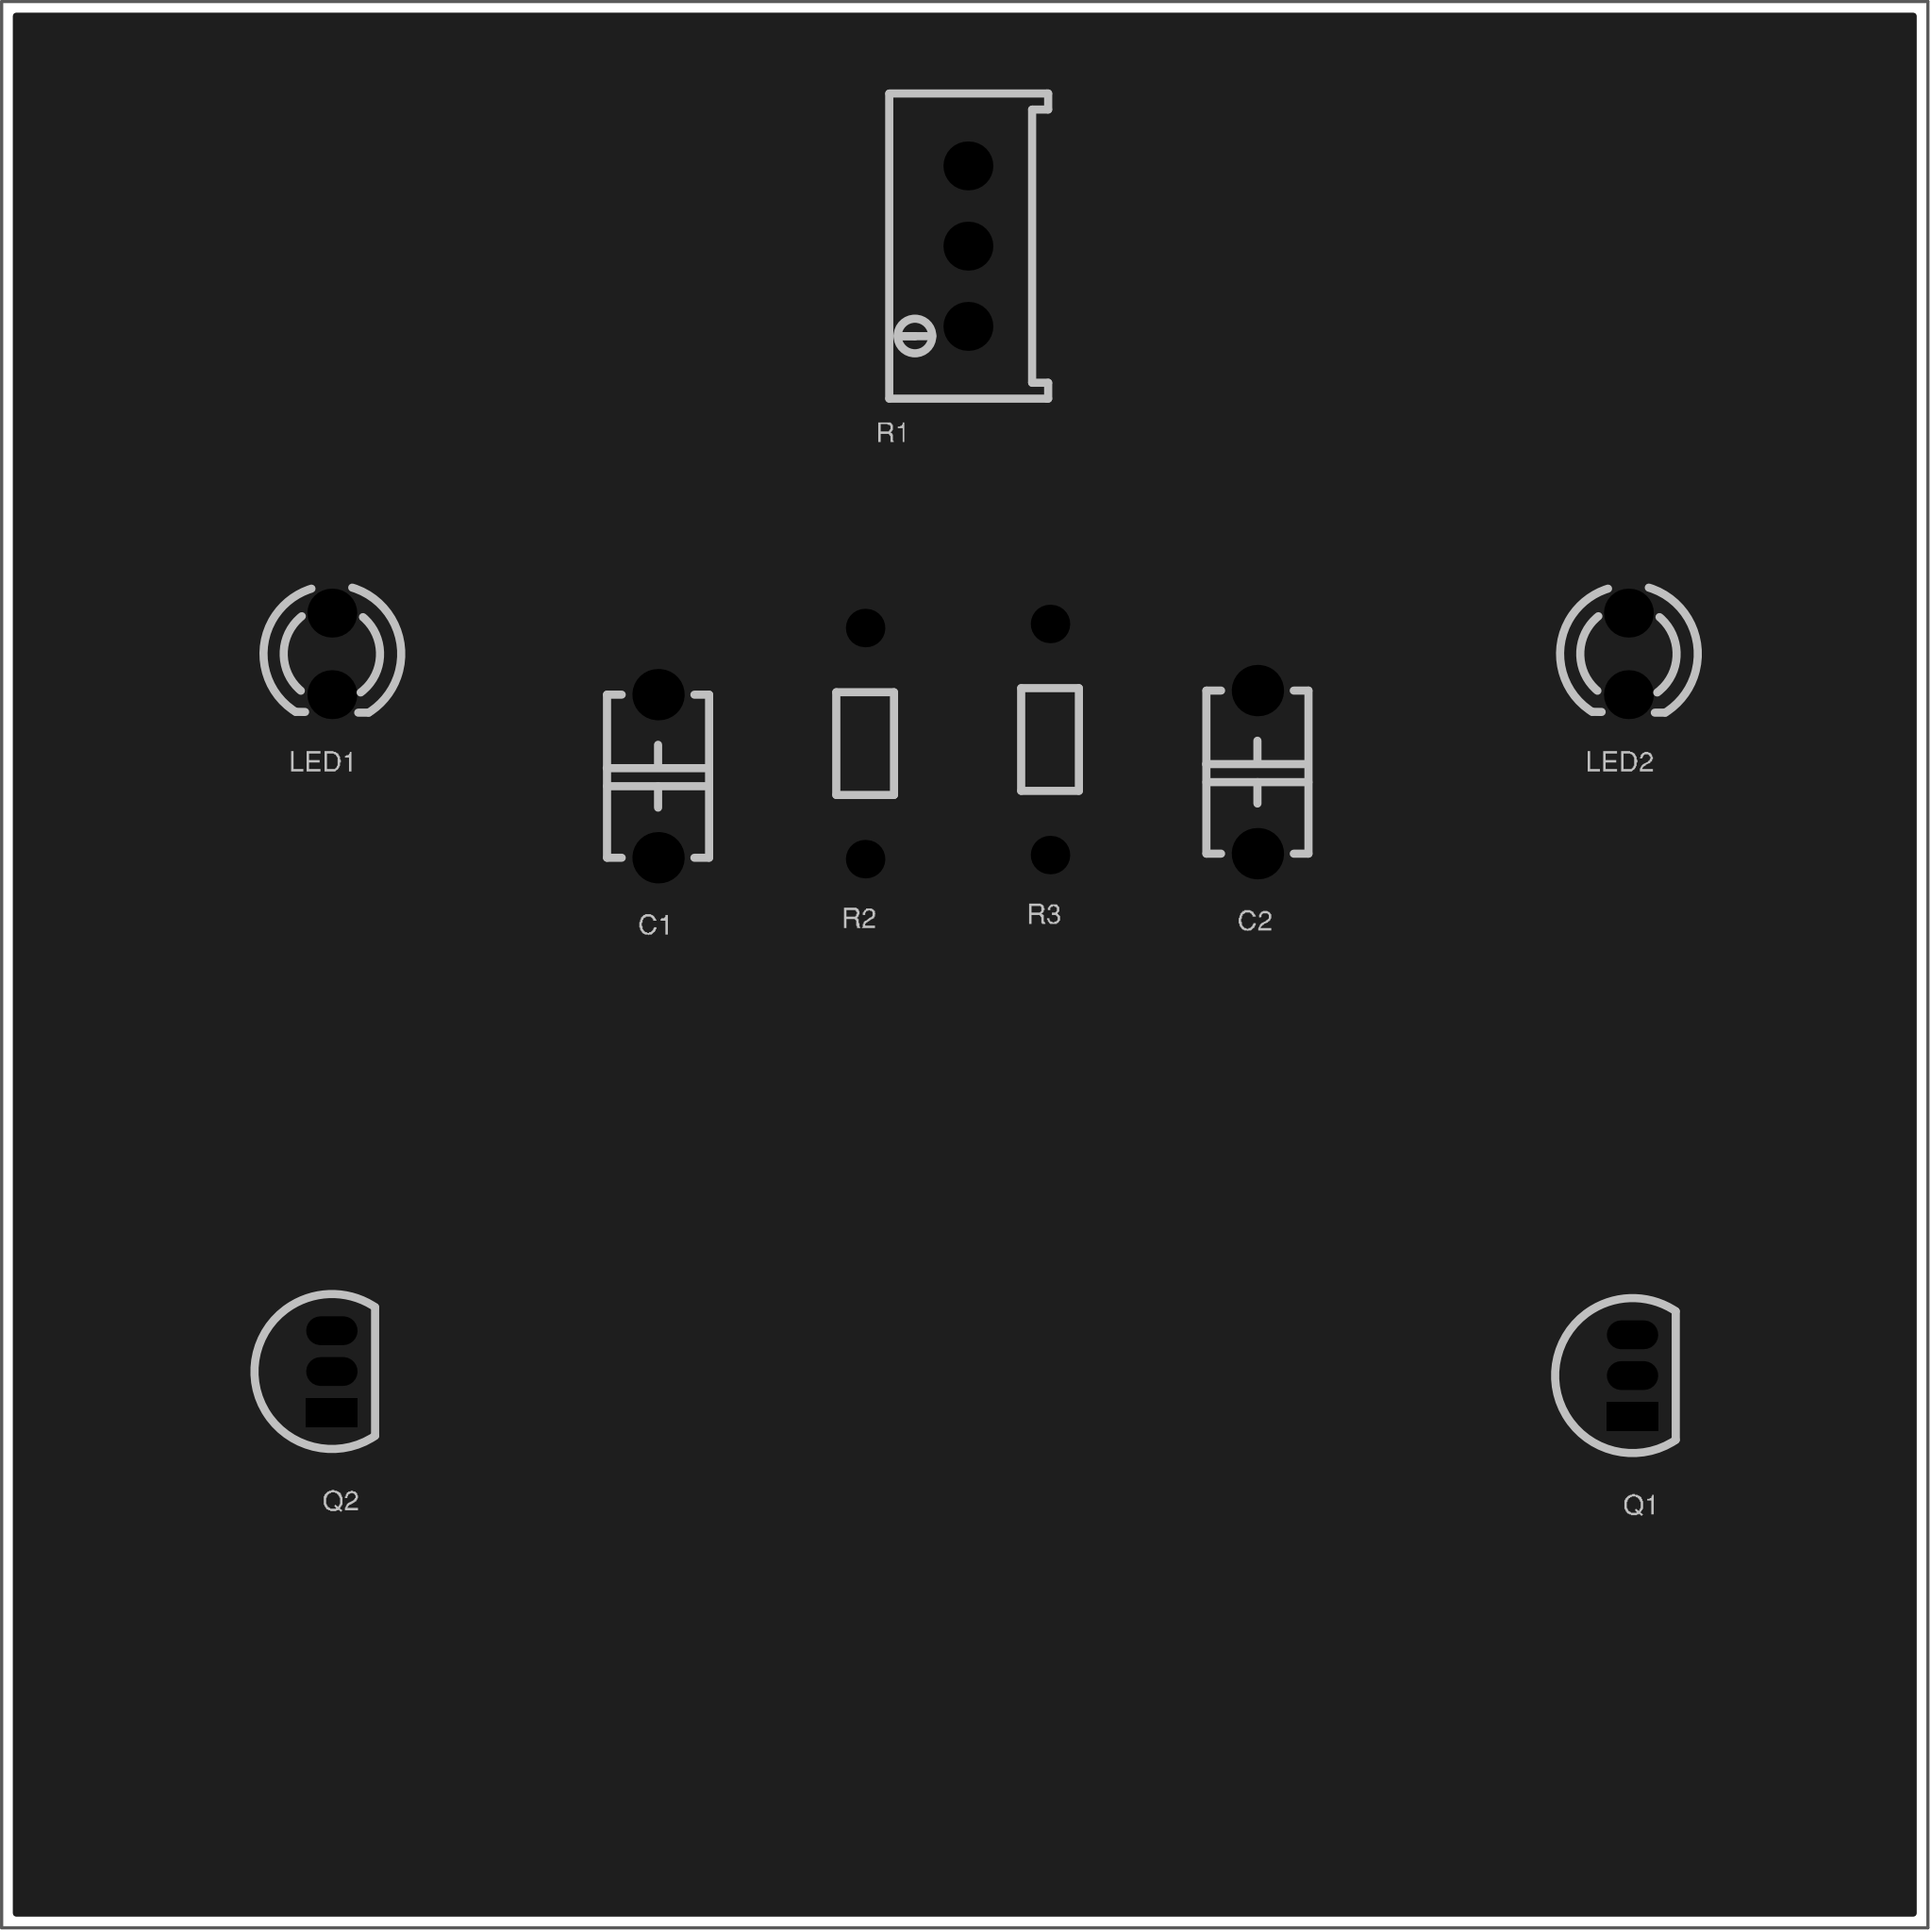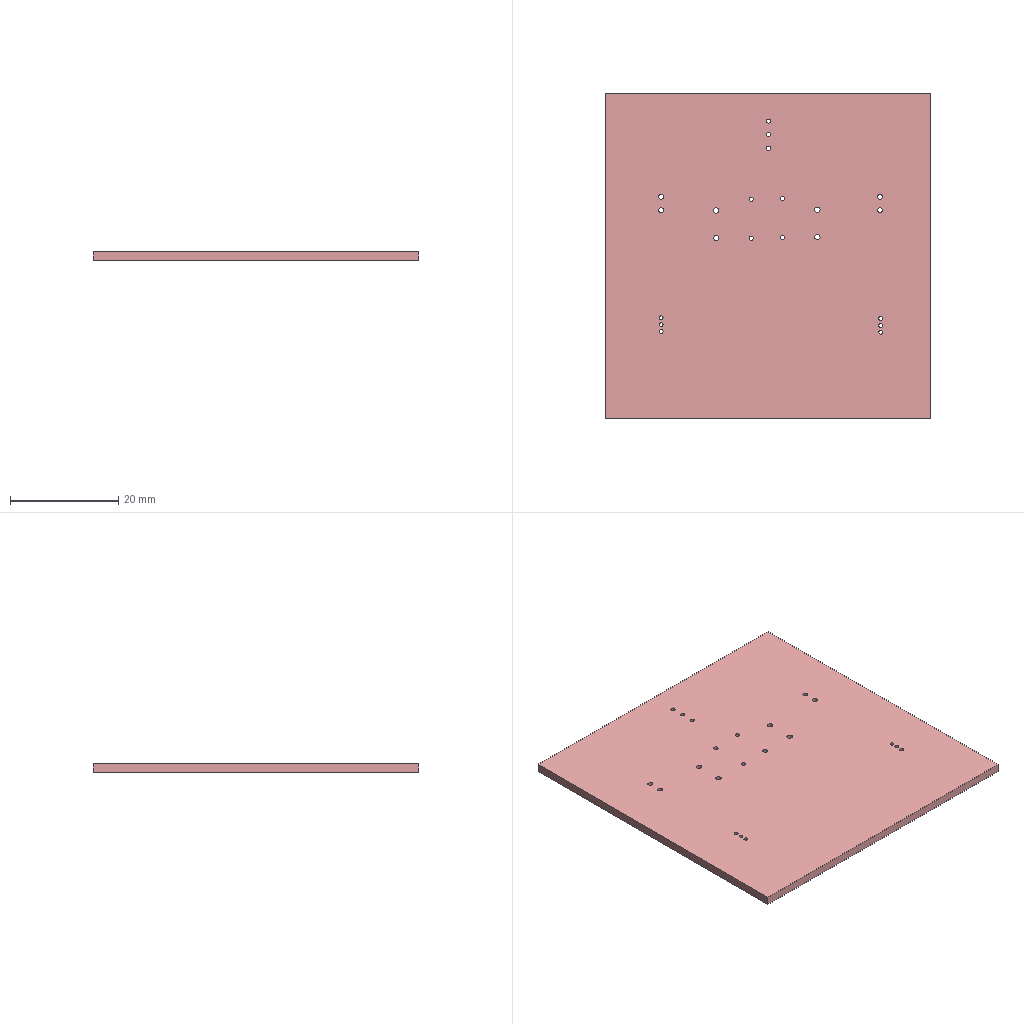Circuit board layout | Altium Designer | box 60 x 60 x 1.6 mm
Layer stack:
# Altium Designer layer stack of  (unit mm; dielectric type: 0 none, 1 core, 2 prepreg, 3 surface material)
index,name,kind,layer,copper_thickness_mm,dielectric_type,dielectric_thickness_mm,dielectric_material,dielectric_constant
0,Top Paste Mask Layer,other,,,,,,
1,Top Silkscreen Layer,other,,,,,,
2,Top Solder Mask Layer,dielectric,,,3,0.01,,3.3
3,Top Layer,copper,Top Layer,0.035,,,,
4,Dielectric1,dielectric,,,3,1.51,FR4,4.5
5,Bottom Layer,copper,Bottom Layer,0.035,,,,
6,Bottom Solder Mask Layer,dielectric,,,3,0.01,,3.3
7,Bottom Silkscreen Layer,other,,,,,,
8,Bottom Paste Mask Layer,other,,,,,,
# drill layer pairs: low layer,high layer
drill_pair,Top Layer,Bottom Layer
Part placement:
Designator,Comment,Layer,Footprint,Center-X(mm),Center-Y(mm),Rotation
C1,100uF,TopLayer,CAP-TH_L5.1-W3.2-P5.08-D0.50,96.647,112.07,270
C2,100uF,TopLayer,CAP-TH_L5.1-W3.2-P5.08-D0.50,115.316,112.197,270
LED1,,TopLayer,LED_TH-3mm,86.487,115.88,270
LED2,,TopLayer,LED_TH-3mm,126.873,115.88,270
Q1,,TopLayer,S8050_TO_92,127,93.401,90
Q2,,TopLayer,S8050_TO_92,86.487,93.528,90
R1,10k,TopLayer,R_3296,106.299,128.58,90
R2,10k,TopLayer,Res_1/8W,103.097,113.086,90
R3,10k,TopLayer,Res_1/8W,108.856,113.213,90
Pad and via stacks:
# Altium Designer via and pad stacks of  (unit mm). Each distinct definition once, with the count of objects using it.
# via: kind,start_layer,end_layer,hole_mm,diameter_mm,mode(0 simple;1 top-mid-bottom;2 full stack),diameter_per_layer,count,example_net
# pad: kind,layer,hole_mm,hole_type(0 round;1 square;2 slot),plating,top_size,top_shape(1 round;2 rect;3 octagon;9 rounded rect),mid_size,bottom_size,mode,footprint,size_per_layer,count,example
pad,Multi-Layer,1,0,plated,1.6x1.6,1,1.6x1.6,1.6x1.6,0,CAP-TH_L5.1-W3.2-P5.08-D0.50,,4,C1.2
pad,Multi-Layer,0.9144,0,plated,1.524x1.524,1,1.524x1.524,1.524x1.524,0,LED_TH-3mm,,4,LED1.1
pad,Multi-Layer,0.701,0,plated,0.8992x1.6,2,0.8992x1.6,0.8992x1.6,0,S8050_TO_92,,2,Q1.1
pad,Multi-Layer,0.701,0,plated,0.8992x1.6,1,0.8992x1.6,0.8992x1.6,0,S8050_TO_92,,4,Q1.2
pad,Multi-Layer,0.762,0,plated,1.524x1.524,1,1.524x1.524,1.524x1.524,0,R_3296,,3,R1.2
pad,Multi-Layer,0.8001,0,plated,1.199x1.199,1,1.199x1.199,1.199x1.199,0,Res_1/8W,,4,R2.1
Copper pours:
name,layer,net,type(0 solid;1 hatched;2 none)
Top Layer-GND,Top Layer,GND,0
Bottom Layer-GND,Bottom Layer,GND,0
Design rules, without the lines most boards share:
# Altium Designer design rules of  (exported by Altium Designer, unit mm)
# columns: name | kind | enabled | priority | scope1 | scope2 | descriptor | typed fields (field=value)
creepage | 65 | enabled | 1 | All | All | Creepage Distance Constraint =(0mil) (All),(All) |
copperThickness1oz_2 | 2 | enabled | 2 | All | All | Width Constraint (Min=13.8mil) (Max=100mil) (Preferred=13.8mil) (All) |
viaSize | 11 | enabled | 1 | All | All | Routing Via (MinHoleWidth=11.811mil) (MaxHoleWidth=248.031mil) (PreferredHoleWidth=11.811mil) (MinWidth=19.685mil) (MaxWidth=393.701mil) (PreferedWidth=19.685mil) (All) | via_min_hole=0.3 via_max_hole=6.3 via_preferred_diameter=0.5 via_preferred_hole=0.3